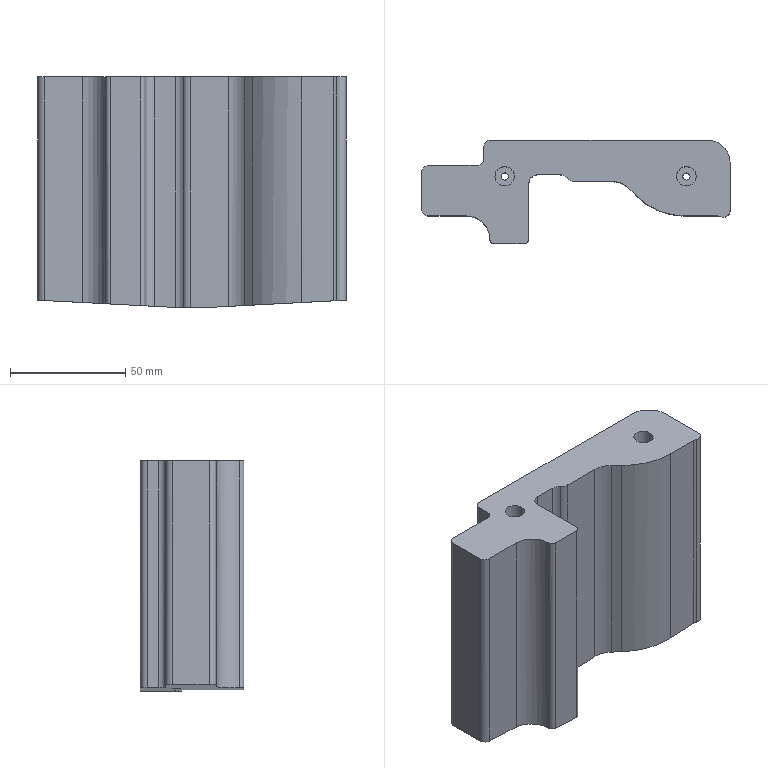Part | STEP file | lll_id238_x_t | 1 solid | 37 faces | box 134 x 45 x 100 mm | volume 341520 mm3 | cylinder 19 | plane 18 | commonest cylinder face diameters 6 x6 3.1 x2 4 x2 8 x2 8.506 x2 20 x2
STEP:
#1=CARTESIAN_POINT('',(1111.,-25.501,-7.5));
#2=VERTEX_POINT('',#1);
#3=CARTESIAN_POINT('',(1111.,-7.5,-7.5));
#4=VERTEX_POINT('',#3);
#5=CARTESIAN_POINT('',(1111.,-7.5,-7.5));
#6=DIRECTION('',(0.,1.,0.));
#7=VECTOR('',#6,1.);
#8=LINE('',#5,#7);
#9=EDGE_CURVE('',#2,#4,#8,.T.);
#10=ORIENTED_EDGE('',*,*,#9,.F.);
#11=CARTESIAN_POINT('',(1100.313,-25.498,-7.5));
#12=VERTEX_POINT('',#11);
#13=CARTESIAN_POINT('',(1065.507,-25.488,-7.5));
#14=DIRECTION('',(-1.,0.0002888,0.));
#15=VECTOR('',#14,1.);
#16=LINE('',#13,#15);
#17=EDGE_CURVE('',#2,#12,#16,.T.);
#18=ORIENTED_EDGE('',*,*,#17,.T.);
#19=CARTESIAN_POINT('',(1097.128,-23.983,-7.5));
#20=VERTEX_POINT('',#19);
#21=CARTESIAN_POINT('',(1100.299,-21.422,-7.5));
#22=DIRECTION('',(0.,0.,1.));
#23=DIRECTION('',(1.,0.,0.));
#24=AXIS2_PLACEMENT_3D('',#21,#22,#23);
#25=CIRCLE('',#24,4.076);
#26=EDGE_CURVE('',#20,#12,#25,.T.);
#27=ORIENTED_EDGE('',*,*,#26,.F.);
#28=CARTESIAN_POINT('',(1094.017,-22.497,-7.5));
#29=VERTEX_POINT('',#28);
#30=CARTESIAN_POINT('',(1094.016,-26.497,-7.5));
#31=DIRECTION('',(0.,0.,-1.));
#32=DIRECTION('',(1.,0.,0.));
#33=AXIS2_PLACEMENT_3D('',#30,#31,#32);
#34=CIRCLE('',#33,4.);
#35=EDGE_CURVE('',#29,#20,#34,.T.);
#36=ORIENTED_EDGE('',*,*,#35,.F.);
#37=CARTESIAN_POINT('',(1091.,-22.496,-7.5));
#38=VERTEX_POINT('',#37);
#39=CARTESIAN_POINT('',(1065.505,-22.492,-7.5));
#40=DIRECTION('',(-1.,0.0001728,0.));
#41=VECTOR('',#40,1.);
#42=LINE('',#39,#41);
#43=EDGE_CURVE('',#29,#38,#42,.T.);
#44=ORIENTED_EDGE('',*,*,#43,.T.);
#45=CARTESIAN_POINT('',(1091.,-7.5,-7.5));
#46=VERTEX_POINT('',#45);
#47=CARTESIAN_POINT('',(1091.,-7.5,-7.5));
#48=DIRECTION('',(0.,-1.,0.));
#49=VECTOR('',#48,1.);
#50=LINE('',#47,#49);
#51=EDGE_CURVE('',#46,#38,#50,.T.);
#52=ORIENTED_EDGE('',*,*,#51,.F.);
#53=CARTESIAN_POINT('',(1065.5,-7.5,-7.5));
#54=DIRECTION('',(-1.,0.,0.));
#55=VECTOR('',#54,1.);
#56=LINE('',#53,#55);
#57=EDGE_CURVE('',#4,#46,#56,.T.);
#58=ORIENTED_EDGE('',*,*,#57,.F.);
#59=EDGE_LOOP('',(#10,#18,#27,#36,#44,#52,#58));
#60=FACE_OUTER_BOUND('',#59,.T.);
#61=CARTESIAN_POINT('',(1065.5,-50.5,-7.5));
#62=DIRECTION('',(0.,0.,1.));
#63=DIRECTION('',(-1.,0.,0.));
#64=AXIS2_PLACEMENT_3D('',#61,#62,#63);
#65=PLANE('',#64);
#66=ADVANCED_FACE('',(#60),#65,.F.);
#67=CARTESIAN_POINT('',(1068.45,-23.25,30.747));
#68=VERTEX_POINT('',#67);
#69=CARTESIAN_POINT('',(1070.,-23.25,30.747));
#70=DIRECTION('',(0.,0.,1.));
#71=DIRECTION('',(-1.,0.,0.));
#72=AXIS2_PLACEMENT_3D('',#69,#70,#71);
#73=CIRCLE('',#72,1.55);
#74=EDGE_CURVE('',#68,#68,#73,.T.);
#75=ORIENTED_EDGE('',*,*,#74,.T.);
#76=EDGE_LOOP('',(#75));
#77=FACE_BOUND('',#76,.T.);
#78=CARTESIAN_POINT('',(1071.55,-23.25,-6.476));
#79=VERTEX_POINT('',#78);
#80=CARTESIAN_POINT('',(1070.,-23.25,-6.395));
#81=DIRECTION('',(-0.05256,0.,-0.9986));
#82=DIRECTION('',(0.9986,0.,-0.05256));
#83=AXIS2_PLACEMENT_3D('',#80,#81,#82);
#84=ELLIPSE('',#83,1.552,1.55);
#85=EDGE_CURVE('',#79,#79,#84,.T.);
#86=ORIENTED_EDGE('',*,*,#85,.T.);
#87=EDGE_LOOP('',(#86));
#88=FACE_BOUND('',#87,.T.);
#89=CARTESIAN_POINT('',(1070.,-23.25,37.747));
#90=DIRECTION('',(0.,0.,-1.));
#91=DIRECTION('',(-1.,0.,0.));
#92=AXIS2_PLACEMENT_3D('',#89,#90,#91);
#93=CYLINDRICAL_SURFACE('',#92,1.55);
#94=ADVANCED_FACE('',(#77,#88),#93,.F.);
#95=CARTESIAN_POINT('',(1147.45,-23.25,30.747));
#96=VERTEX_POINT('',#95);
#97=CARTESIAN_POINT('',(1149.,-23.25,30.747));
#98=DIRECTION('',(0.,0.,1.));
#99=DIRECTION('',(-1.,0.,0.));
#100=AXIS2_PLACEMENT_3D('',#97,#98,#99);
#101=CIRCLE('',#100,1.55);
#102=EDGE_CURVE('',#96,#96,#101,.T.);
#103=ORIENTED_EDGE('',*,*,#102,.T.);
#104=EDGE_LOOP('',(#103));
#105=FACE_BOUND('',#104,.T.);
#106=CARTESIAN_POINT('',(1147.45,-23.25,-5.582));
#107=VERTEX_POINT('',#106);
#108=CARTESIAN_POINT('',(1149.,-23.25,-5.5));
#109=DIRECTION('',(0.05256,0.,-0.9986));
#110=DIRECTION('',(-0.9986,0.,-0.05256));
#111=AXIS2_PLACEMENT_3D('',#108,#109,#110);
#112=ELLIPSE('',#111,1.552,1.55);
#113=EDGE_CURVE('',#107,#107,#112,.T.);
#114=ORIENTED_EDGE('',*,*,#113,.T.);
#115=EDGE_LOOP('',(#114));
#116=FACE_BOUND('',#115,.T.);
#117=CARTESIAN_POINT('',(1149.,-23.25,37.747));
#118=DIRECTION('',(0.,0.,-1.));
#119=DIRECTION('',(-1.,0.,0.));
#120=AXIS2_PLACEMENT_3D('',#117,#118,#119);
#121=CYLINDRICAL_SURFACE('',#120,1.55);
#122=ADVANCED_FACE('',(#105,#116),#121,.F.);
#123=CARTESIAN_POINT('',(1116.863,-25.503,92.5));
#124=VERTEX_POINT('',#123);
#125=CARTESIAN_POINT('',(1100.313,-25.498,92.5));
#126=VERTEX_POINT('',#125);
#127=CARTESIAN_POINT('',(1065.507,-25.488,92.5));
#128=DIRECTION('',(-1.,0.0002888,0.));
#129=VECTOR('',#128,1.);
#130=LINE('',#127,#129);
#131=EDGE_CURVE('',#124,#126,#130,.T.);
#132=ORIENTED_EDGE('',*,*,#131,.F.);
#133=CARTESIAN_POINT('',(1123.932,-28.432,92.5));
#134=VERTEX_POINT('',#133);
#135=CARTESIAN_POINT('',(1116.86,-35.503,92.5));
#136=DIRECTION('',(0.,0.,1.));
#137=DIRECTION('',(1.,0.,0.));
#138=AXIS2_PLACEMENT_3D('',#135,#136,#137);
#139=CIRCLE('',#138,10.);
#140=EDGE_CURVE('',#134,#124,#139,.T.);
#141=ORIENTED_EDGE('',*,*,#140,.F.);
#142=CARTESIAN_POINT('',(1127.213,-31.713,92.5));
#143=VERTEX_POINT('',#142);
#144=CARTESIAN_POINT('',(1105.75,-10.25,92.5));
#145=DIRECTION('',(0.7071,-0.7071,0.));
#146=VECTOR('',#145,1.);
#147=LINE('',#144,#146);
#148=EDGE_CURVE('',#134,#143,#147,.T.);
#149=ORIENTED_EDGE('',*,*,#148,.T.);
#150=CARTESIAN_POINT('',(1148.426,-40.5,92.5));
#151=VERTEX_POINT('',#150);
#152=CARTESIAN_POINT('',(1148.426,-10.502,92.5));
#153=DIRECTION('',(0.,0.,1.));
#154=DIRECTION('',(1.,0.,0.));
#155=AXIS2_PLACEMENT_3D('',#152,#153,#154);
#156=CIRCLE('',#155,29.998);
#157=EDGE_CURVE('',#143,#151,#156,.T.);
#158=ORIENTED_EDGE('',*,*,#157,.T.);
#159=CARTESIAN_POINT('',(1162.602,-40.5,92.5));
#160=VERTEX_POINT('',#159);
#161=CARTESIAN_POINT('',(1065.5,-40.5,92.5));
#162=DIRECTION('',(1.,0.,0.));
#163=VECTOR('',#162,1.);
#164=LINE('',#161,#163);
#165=EDGE_CURVE('',#151,#160,#164,.T.);
#166=ORIENTED_EDGE('',*,*,#165,.T.);
#167=CARTESIAN_POINT('',(1163.801,-40.75,92.5));
#168=VERTEX_POINT('',#167);
#169=CARTESIAN_POINT('',(1162.602,-43.5,92.5));
#170=DIRECTION('',(0.,0.,-1.));
#171=DIRECTION('',(1.,0.,0.));
#172=AXIS2_PLACEMENT_3D('',#169,#170,#171);
#173=CIRCLE('',#172,3.);
#174=EDGE_CURVE('',#160,#168,#173,.T.);
#175=ORIENTED_EDGE('',*,*,#174,.T.);
#176=CARTESIAN_POINT('',(1168.,-38.,92.5));
#177=VERTEX_POINT('',#176);
#178=CARTESIAN_POINT('',(1165.,-38.,92.5));
#179=DIRECTION('',(0.,0.,1.));
#180=DIRECTION('',(1.,0.,0.));
#181=AXIS2_PLACEMENT_3D('',#178,#179,#180);
#182=CIRCLE('',#181,3.);
#183=EDGE_CURVE('',#168,#177,#182,.T.);
#184=ORIENTED_EDGE('',*,*,#183,.T.);
#185=CARTESIAN_POINT('',(1168.,-17.5,92.5));
#186=VERTEX_POINT('',#185);
#187=CARTESIAN_POINT('',(1168.,-50.5,92.5));
#188=DIRECTION('',(0.,-1.,0.));
#189=VECTOR('',#188,1.);
#190=LINE('',#187,#189);
#191=EDGE_CURVE('',#186,#177,#190,.T.);
#192=ORIENTED_EDGE('',*,*,#191,.F.);
#193=CARTESIAN_POINT('',(1158.,-7.5,92.5));
#194=VERTEX_POINT('',#193);
#195=CARTESIAN_POINT('',(1158.,-17.5,92.5));
#196=DIRECTION('',(0.,0.,1.));
#197=DIRECTION('',(1.,0.,0.));
#198=AXIS2_PLACEMENT_3D('',#195,#196,#197);
#199=CIRCLE('',#198,10.);
#200=EDGE_CURVE('',#186,#194,#199,.T.);
#201=ORIENTED_EDGE('',*,*,#200,.T.);
#202=CARTESIAN_POINT('',(1064.,-7.5,92.5));
#203=VERTEX_POINT('',#202);
#204=CARTESIAN_POINT('',(1065.5,-7.5,92.5));
#205=DIRECTION('',(-1.,0.,0.));
#206=VECTOR('',#205,1.);
#207=LINE('',#204,#206);
#208=EDGE_CURVE('',#194,#203,#207,.T.);
#209=ORIENTED_EDGE('',*,*,#208,.T.);
#210=CARTESIAN_POINT('',(1061.,-10.5,92.5));
#211=VERTEX_POINT('',#210);
#212=CARTESIAN_POINT('',(1064.,-10.5,92.5));
#213=DIRECTION('',(0.,0.,-1.));
#214=DIRECTION('',(1.,0.,0.));
#215=AXIS2_PLACEMENT_3D('',#212,#213,#214);
#216=CIRCLE('',#215,3.);
#217=EDGE_CURVE('',#211,#203,#216,.T.);
#218=ORIENTED_EDGE('',*,*,#217,.F.);
#219=CARTESIAN_POINT('',(1061.,-15.5,92.5));
#220=VERTEX_POINT('',#219);
#221=CARTESIAN_POINT('',(1061.,-50.5,92.5));
#222=DIRECTION('',(0.,1.,0.));
#223=VECTOR('',#222,1.);
#224=LINE('',#221,#223);
#225=EDGE_CURVE('',#220,#211,#224,.T.);
#226=ORIENTED_EDGE('',*,*,#225,.F.);
#227=CARTESIAN_POINT('',(1058.,-18.5,92.5));
#228=VERTEX_POINT('',#227);
#229=CARTESIAN_POINT('',(1058.,-15.5,92.5));
#230=DIRECTION('',(0.,0.,-1.));
#231=DIRECTION('',(1.,0.,0.));
#232=AXIS2_PLACEMENT_3D('',#229,#230,#231);
#233=CIRCLE('',#232,3.);
#234=EDGE_CURVE('',#220,#228,#233,.T.);
#235=ORIENTED_EDGE('',*,*,#234,.T.);
#236=CARTESIAN_POINT('',(1037.,-18.5,92.5));
#237=VERTEX_POINT('',#236);
#238=CARTESIAN_POINT('',(1065.5,-18.5,92.5));
#239=DIRECTION('',(1.,0.,0.));
#240=VECTOR('',#239,1.);
#241=LINE('',#238,#240);
#242=EDGE_CURVE('',#237,#228,#241,.T.);
#243=ORIENTED_EDGE('',*,*,#242,.F.);
#244=CARTESIAN_POINT('',(1034.,-21.5,92.5));
#245=VERTEX_POINT('',#244);
#246=CARTESIAN_POINT('',(1037.,-21.5,92.5));
#247=DIRECTION('',(0.,0.,1.));
#248=DIRECTION('',(1.,0.,0.));
#249=AXIS2_PLACEMENT_3D('',#246,#247,#248);
#250=CIRCLE('',#249,3.);
#251=EDGE_CURVE('',#237,#245,#250,.T.);
#252=ORIENTED_EDGE('',*,*,#251,.T.);
#253=CARTESIAN_POINT('',(1034.,-37.5,92.5));
#254=VERTEX_POINT('',#253);
#255=CARTESIAN_POINT('',(1034.,-50.5,92.5));
#256=DIRECTION('',(0.,1.,0.));
#257=VECTOR('',#256,1.);
#258=LINE('',#255,#257);
#259=EDGE_CURVE('',#254,#245,#258,.T.);
#260=ORIENTED_EDGE('',*,*,#259,.F.);
#261=CARTESIAN_POINT('',(1037.,-40.5,92.5));
#262=VERTEX_POINT('',#261);
#263=CARTESIAN_POINT('',(1037.,-37.5,92.5));
#264=DIRECTION('',(0.,0.,-1.));
#265=DIRECTION('',(1.,0.,0.));
#266=AXIS2_PLACEMENT_3D('',#263,#264,#265);
#267=CIRCLE('',#266,3.);
#268=EDGE_CURVE('',#262,#254,#267,.T.);
#269=ORIENTED_EDGE('',*,*,#268,.F.);
#270=CARTESIAN_POINT('',(1053.5,-40.5,92.5));
#271=VERTEX_POINT('',#270);
#272=CARTESIAN_POINT('',(1065.5,-40.5,92.5));
#273=DIRECTION('',(1.,0.,0.));
#274=VECTOR('',#273,1.);
#275=LINE('',#272,#274);
#276=EDGE_CURVE('',#262,#271,#275,.T.);
#277=ORIENTED_EDGE('',*,*,#276,.T.);
#278=CARTESIAN_POINT('',(1063.5,-50.5,92.5));
#279=VERTEX_POINT('',#278);
#280=CARTESIAN_POINT('',(1053.499,-50.501,92.5));
#281=DIRECTION('',(0.,0.,-1.));
#282=DIRECTION('',(1.,0.,0.));
#283=AXIS2_PLACEMENT_3D('',#280,#281,#282);
#284=CIRCLE('',#283,10.001);
#285=EDGE_CURVE('',#271,#279,#284,.T.);
#286=ORIENTED_EDGE('',*,*,#285,.T.);
#287=CARTESIAN_POINT('',(1065.5,-52.5,92.5));
#288=VERTEX_POINT('',#287);
#289=CARTESIAN_POINT('',(1065.5,-50.5,92.5));
#290=DIRECTION('',(0.,0.,1.));
#291=DIRECTION('',(1.,0.,0.));
#292=AXIS2_PLACEMENT_3D('',#289,#290,#291);
#293=CIRCLE('',#292,2.);
#294=EDGE_CURVE('',#279,#288,#293,.T.);
#295=ORIENTED_EDGE('',*,*,#294,.T.);
#296=CARTESIAN_POINT('',(1078.51,-52.5,92.5));
#297=VERTEX_POINT('',#296);
#298=CARTESIAN_POINT('',(1065.5,-52.5,92.5));
#299=DIRECTION('',(-1.,0.,0.));
#300=VECTOR('',#299,1.);
#301=LINE('',#298,#300);
#302=EDGE_CURVE('',#297,#288,#301,.T.);
#303=ORIENTED_EDGE('',*,*,#302,.F.);
#304=CARTESIAN_POINT('',(1080.51,-50.5,92.5));
#305=VERTEX_POINT('',#304);
#306=CARTESIAN_POINT('',(1078.51,-50.5,92.5));
#307=DIRECTION('',(0.,0.,-1.));
#308=DIRECTION('',(1.,0.,0.));
#309=AXIS2_PLACEMENT_3D('',#306,#307,#308);
#310=CIRCLE('',#309,2.);
#311=EDGE_CURVE('',#305,#297,#310,.T.);
#312=ORIENTED_EDGE('',*,*,#311,.F.);
#313=CARTESIAN_POINT('',(1080.512,-26.495,92.5));
#314=VERTEX_POINT('',#313);
#315=CARTESIAN_POINT('',(1080.51,-50.501,92.5));
#316=DIRECTION('',(0.00006142,1.,0.));
#317=VECTOR('',#316,1.);
#318=LINE('',#315,#317);
#319=EDGE_CURVE('',#305,#314,#318,.T.);
#320=ORIENTED_EDGE('',*,*,#319,.T.);
#321=CARTESIAN_POINT('',(1084.513,-22.495,92.5));
#322=VERTEX_POINT('',#321);
#323=CARTESIAN_POINT('',(1084.512,-26.495,92.5));
#324=DIRECTION('',(0.,0.,1.));
#325=DIRECTION('',(1.,0.,0.));
#326=AXIS2_PLACEMENT_3D('',#323,#324,#325);
#327=CIRCLE('',#326,4.);
#328=EDGE_CURVE('',#322,#314,#327,.T.);
#329=ORIENTED_EDGE('',*,*,#328,.F.);
#330=CARTESIAN_POINT('',(1094.017,-22.497,92.5));
#331=VERTEX_POINT('',#330);
#332=CARTESIAN_POINT('',(1065.505,-22.492,92.5));
#333=DIRECTION('',(1.,-0.0001728,0.));
#334=VECTOR('',#333,1.);
#335=LINE('',#332,#334);
#336=EDGE_CURVE('',#322,#331,#335,.T.);
#337=ORIENTED_EDGE('',*,*,#336,.T.);
#338=CARTESIAN_POINT('',(1097.128,-23.983,92.5));
#339=VERTEX_POINT('',#338);
#340=CARTESIAN_POINT('',(1094.016,-26.497,92.5));
#341=DIRECTION('',(0.,0.,1.));
#342=DIRECTION('',(1.,0.,0.));
#343=AXIS2_PLACEMENT_3D('',#340,#341,#342);
#344=CIRCLE('',#343,4.);
#345=EDGE_CURVE('',#339,#331,#344,.T.);
#346=ORIENTED_EDGE('',*,*,#345,.F.);
#347=CARTESIAN_POINT('',(1100.299,-21.422,92.5));
#348=DIRECTION('',(0.,0.,1.));
#349=DIRECTION('',(1.,0.,0.));
#350=AXIS2_PLACEMENT_3D('',#347,#348,#349);
#351=CIRCLE('',#350,4.076);
#352=EDGE_CURVE('',#339,#126,#351,.T.);
#353=ORIENTED_EDGE('',*,*,#352,.T.);
#354=EDGE_LOOP('',(#132,#141,#149,#158,#166,#175,#184,#192,#201,#209,#218,#226,#235,#243,#252,#260,#269,#277,#286,#295,#303,#312,#320,#329,#337,#346,#353));
#355=FACE_BOUND('',#354,.T.);
#356=CARTESIAN_POINT('',(1153.253,-23.25,92.5));
#357=VERTEX_POINT('',#356);
#358=CARTESIAN_POINT('',(1149.,-23.25,92.5));
#359=DIRECTION('',(0.,0.,-1.));
#360=DIRECTION('',(1.,0.,0.));
#361=AXIS2_PLACEMENT_3D('',#358,#359,#360);
#362=CIRCLE('',#361,4.253);
#363=EDGE_CURVE('',#357,#357,#362,.T.);
#364=ORIENTED_EDGE('',*,*,#363,.T.);
#365=EDGE_LOOP('',(#364));
#366=FACE_BOUND('',#365,.T.);
#367=CARTESIAN_POINT('',(1074.253,-23.25,92.5));
#368=VERTEX_POINT('',#367);
#369=CARTESIAN_POINT('',(1070.,-23.25,92.5));
#370=DIRECTION('',(0.,0.,-1.));
#371=DIRECTION('',(1.,0.,0.));
#372=AXIS2_PLACEMENT_3D('',#369,#370,#371);
#373=CIRCLE('',#372,4.253);
#374=EDGE_CURVE('',#368,#368,#373,.T.);
#375=ORIENTED_EDGE('',*,*,#374,.T.);
#376=EDGE_LOOP('',(#375));
#377=FACE_BOUND('',#376,.T.);
#378=CARTESIAN_POINT('',(1065.5,-50.5,92.5));
#379=DIRECTION('',(0.,0.,1.));
#380=DIRECTION('',(-1.,0.,0.));
#381=AXIS2_PLACEMENT_3D('',#378,#379,#380);
#382=PLANE('',#381);
#383=ADVANCED_FACE('',(#355,#366,#377),#382,.T.);
#384=ORIENTED_EDGE('',*,*,#363,.F.);
#385=EDGE_LOOP('',(#384));
#386=FACE_BOUND('',#385,.T.);
#387=CARTESIAN_POINT('',(1144.747,-23.25,30.747));
#388=VERTEX_POINT('',#387);
#389=CARTESIAN_POINT('',(1149.,-23.25,30.747));
#390=DIRECTION('',(0.,0.,-1.));
#391=DIRECTION('',(-1.,0.,0.));
#392=AXIS2_PLACEMENT_3D('',#389,#390,#391);
#393=CIRCLE('',#392,4.253);
#394=EDGE_CURVE('',#388,#388,#393,.T.);
#395=ORIENTED_EDGE('',*,*,#394,.T.);
#396=EDGE_LOOP('',(#395));
#397=FACE_BOUND('',#396,.T.);
#398=CARTESIAN_POINT('',(1149.,-23.25,94.5));
#399=DIRECTION('',(0.,0.,-1.));
#400=DIRECTION('',(1.,0.,0.));
#401=AXIS2_PLACEMENT_3D('',#398,#399,#400);
#402=CYLINDRICAL_SURFACE('',#401,4.253);
#403=ADVANCED_FACE('',(#386,#397),#402,.F.);
#404=ORIENTED_EDGE('',*,*,#374,.F.);
#405=EDGE_LOOP('',(#404));
#406=FACE_BOUND('',#405,.T.);
#407=CARTESIAN_POINT('',(1065.747,-23.25,30.747));
#408=VERTEX_POINT('',#407);
#409=CARTESIAN_POINT('',(1070.,-23.25,30.747));
#410=DIRECTION('',(0.,0.,-1.));
#411=DIRECTION('',(-1.,0.,0.));
#412=AXIS2_PLACEMENT_3D('',#409,#410,#411);
#413=CIRCLE('',#412,4.253);
#414=EDGE_CURVE('',#408,#408,#413,.T.);
#415=ORIENTED_EDGE('',*,*,#414,.T.);
#416=EDGE_LOOP('',(#415));
#417=FACE_BOUND('',#416,.T.);
#418=CARTESIAN_POINT('',(1070.,-23.25,94.5));
#419=DIRECTION('',(0.,0.,-1.));
#420=DIRECTION('',(1.,0.,0.));
#421=AXIS2_PLACEMENT_3D('',#418,#419,#420);
#422=CYLINDRICAL_SURFACE('',#421,4.253);
#423=ADVANCED_FACE('',(#406,#417),#422,.F.);
#424=CARTESIAN_POINT('',(1116.863,-25.503,-7.191));
#425=VERTEX_POINT('',#424);
#426=CARTESIAN_POINT('',(1110.995,-25.501,-7.5));
#427=DIRECTION('',(-0.9986,0.0002884,-0.05256));
#428=VECTOR('',#427,1.);
#429=LINE('',#426,#428);
#430=EDGE_CURVE('',#425,#2,#429,.T.);
#431=ORIENTED_EDGE('',*,*,#430,.T.);
#432=ORIENTED_EDGE('',*,*,#9,.T.);
#433=CARTESIAN_POINT('',(1158.,-7.5,-5.026));
#434=VERTEX_POINT('',#433);
#435=CARTESIAN_POINT('',(1111.,-7.5,-7.5));
#436=DIRECTION('',(0.9986,0.,0.05256));
#437=VECTOR('',#436,1.);
#438=LINE('',#435,#437);
#439=EDGE_CURVE('',#4,#434,#438,.T.);
#440=ORIENTED_EDGE('',*,*,#439,.T.);
#441=CARTESIAN_POINT('',(1168.,-17.5,-4.5));
#442=VERTEX_POINT('',#441);
#443=CARTESIAN_POINT('',(1158.,-17.5,-5.026));
#444=DIRECTION('',(-0.05256,0.,0.9986));
#445=DIRECTION('',(0.9986,0.,0.05256));
#446=AXIS2_PLACEMENT_3D('',#443,#444,#445);
#447=ELLIPSE('',#446,10.014,10.);
#448=EDGE_CURVE('',#442,#434,#447,.T.);
#449=ORIENTED_EDGE('',*,*,#448,.F.);
#450=CARTESIAN_POINT('',(1168.,-38.,-4.5));
#451=VERTEX_POINT('',#450);
#452=CARTESIAN_POINT('',(1168.,-7.5,-4.5));
#453=DIRECTION('',(0.,-1.,0.));
#454=VECTOR('',#453,1.);
#455=LINE('',#452,#454);
#456=EDGE_CURVE('',#442,#451,#455,.T.);
#457=ORIENTED_EDGE('',*,*,#456,.T.);
#458=CARTESIAN_POINT('',(1163.801,-40.75,-4.721));
#459=VERTEX_POINT('',#458);
#460=CARTESIAN_POINT('',(1165.,-38.,-4.658));
#461=DIRECTION('',(-0.05256,0.,0.9986));
#462=DIRECTION('',(0.9986,0.,0.05256));
#463=AXIS2_PLACEMENT_3D('',#460,#461,#462);
#464=ELLIPSE('',#463,3.004,3.);
#465=EDGE_CURVE('',#459,#451,#464,.T.);
#466=ORIENTED_EDGE('',*,*,#465,.F.);
#467=CARTESIAN_POINT('',(1162.602,-40.5,-4.784));
#468=VERTEX_POINT('',#467);
#469=CARTESIAN_POINT('',(1162.602,-43.5,-4.784));
#470=DIRECTION('',(0.05256,0.,-0.9986));
#471=DIRECTION('',(0.9986,0.,0.05256));
#472=AXIS2_PLACEMENT_3D('',#469,#470,#471);
#473=ELLIPSE('',#472,3.004,3.);
#474=EDGE_CURVE('',#468,#459,#473,.T.);
#475=ORIENTED_EDGE('',*,*,#474,.F.);
#476=CARTESIAN_POINT('',(1148.426,-40.5,-5.53));
#477=VERTEX_POINT('',#476);
#478=CARTESIAN_POINT('',(1111.,-40.5,-7.5));
#479=DIRECTION('',(-0.9986,0.,-0.05256));
#480=VECTOR('',#479,1.);
#481=LINE('',#478,#480);
#482=EDGE_CURVE('',#468,#477,#481,.T.);
#483=ORIENTED_EDGE('',*,*,#482,.T.);
#484=CARTESIAN_POINT('',(1127.213,-31.713,-6.647));
#485=VERTEX_POINT('',#484);
#486=CARTESIAN_POINT('',(1148.426,-10.502,-5.53));
#487=DIRECTION('',(0.05256,0.,-0.9986));
#488=DIRECTION('',(0.9986,0.,0.05256));
#489=AXIS2_PLACEMENT_3D('',#486,#487,#488);
#490=ELLIPSE('',#489,30.039,29.998);
#491=EDGE_CURVE('',#477,#485,#490,.T.);
#492=ORIENTED_EDGE('',*,*,#491,.T.);
#493=CARTESIAN_POINT('',(1123.932,-28.432,-6.819));
#494=VERTEX_POINT('',#493);
#495=CARTESIAN_POINT('',(1107.006,-11.506,-7.71));
#496=DIRECTION('',(0.7066,-0.7066,0.03719));
#497=VECTOR('',#496,1.);
#498=LINE('',#495,#497);
#499=EDGE_CURVE('',#494,#485,#498,.T.);
#500=ORIENTED_EDGE('',*,*,#499,.F.);
#501=CARTESIAN_POINT('',(1116.86,-35.503,-7.192));
#502=DIRECTION('',(-0.05256,0.,0.9986));
#503=DIRECTION('',(0.9986,0.,0.05256));
#504=AXIS2_PLACEMENT_3D('',#501,#502,#503);
#505=ELLIPSE('',#504,10.014,10.);
#506=EDGE_CURVE('',#494,#425,#505,.T.);
#507=ORIENTED_EDGE('',*,*,#506,.T.);
#508=EDGE_LOOP('',(#431,#432,#440,#449,#457,#466,#475,#483,#492,#500,#507));
#509=FACE_BOUND('',#508,.T.);
#510=ORIENTED_EDGE('',*,*,#113,.F.);
#511=EDGE_LOOP('',(#510));
#512=FACE_BOUND('',#511,.T.);
#513=CARTESIAN_POINT('',(1111.,-7.5,-7.5));
#514=DIRECTION('',(0.05256,0.,-0.9986));
#515=DIRECTION('',(-0.9986,0.,-0.05256));
#516=AXIS2_PLACEMENT_3D('',#513,#514,#515);
#517=PLANE('',#516);
#518=ADVANCED_FACE('',(#509,#512),#517,.T.);
#519=CARTESIAN_POINT('',(1084.513,-22.495,-7.159));
#520=VERTEX_POINT('',#519);
#521=CARTESIAN_POINT('',(1090.997,-22.496,-7.5));
#522=DIRECTION('',(0.9986,-0.0001725,-0.05256));
#523=VECTOR('',#522,1.);
#524=LINE('',#521,#523);
#525=EDGE_CURVE('',#520,#38,#524,.T.);
#526=ORIENTED_EDGE('',*,*,#525,.F.);
#527=CARTESIAN_POINT('',(1080.512,-26.495,-6.948));
#528=VERTEX_POINT('',#527);
#529=CARTESIAN_POINT('',(1084.512,-26.495,-7.159));
#530=DIRECTION('',(0.05256,0.,0.9986));
#531=DIRECTION('',(-0.9986,0.,0.05256));
#532=AXIS2_PLACEMENT_3D('',#529,#530,#531);
#533=ELLIPSE('',#532,4.006,4.);
#534=EDGE_CURVE('',#520,#528,#533,.T.);
#535=ORIENTED_EDGE('',*,*,#534,.T.);
#536=CARTESIAN_POINT('',(1080.51,-50.5,-6.948));
#537=VERTEX_POINT('',#536);
#538=CARTESIAN_POINT('',(1080.513,-7.499,-6.948));
#539=DIRECTION('',(0.00006142,1.,-0.000003233));
#540=VECTOR('',#539,1.);
#541=LINE('',#538,#540);
#542=EDGE_CURVE('',#537,#528,#541,.T.);
#543=ORIENTED_EDGE('',*,*,#542,.F.);
#544=CARTESIAN_POINT('',(1078.51,-52.5,-6.843));
#545=VERTEX_POINT('',#544);
#546=CARTESIAN_POINT('',(1078.51,-50.5,-6.843));
#547=DIRECTION('',(-0.05256,0.,-0.9986));
#548=DIRECTION('',(-0.9986,0.,0.05256));
#549=AXIS2_PLACEMENT_3D('',#546,#547,#548);
#550=ELLIPSE('',#549,2.003,2.);
#551=EDGE_CURVE('',#537,#545,#550,.T.);
#552=ORIENTED_EDGE('',*,*,#551,.T.);
#553=CARTESIAN_POINT('',(1065.5,-52.5,-6.158));
#554=VERTEX_POINT('',#553);
#555=CARTESIAN_POINT('',(1091.,-52.5,-7.5));
#556=DIRECTION('',(-0.9986,0.,0.05256));
#557=VECTOR('',#556,1.);
#558=LINE('',#555,#557);
#559=EDGE_CURVE('',#545,#554,#558,.T.);
#560=ORIENTED_EDGE('',*,*,#559,.T.);
#561=CARTESIAN_POINT('',(1063.5,-50.5,-6.053));
#562=VERTEX_POINT('',#561);
#563=CARTESIAN_POINT('',(1065.5,-50.5,-6.158));
#564=DIRECTION('',(0.05256,0.,0.9986));
#565=DIRECTION('',(-0.9986,0.,0.05256));
#566=AXIS2_PLACEMENT_3D('',#563,#564,#565);
#567=ELLIPSE('',#566,2.003,2.);
#568=EDGE_CURVE('',#562,#554,#567,.T.);
#569=ORIENTED_EDGE('',*,*,#568,.F.);
#570=CARTESIAN_POINT('',(1053.5,-40.5,-5.526));
#571=VERTEX_POINT('',#570);
#572=CARTESIAN_POINT('',(1053.499,-50.501,-5.526));
#573=DIRECTION('',(-0.05256,0.,-0.9986));
#574=DIRECTION('',(-0.9986,0.,0.05256));
#575=AXIS2_PLACEMENT_3D('',#572,#573,#574);
#576=ELLIPSE('',#575,10.014,10.001);
#577=EDGE_CURVE('',#571,#562,#576,.T.);
#578=ORIENTED_EDGE('',*,*,#577,.F.);
#579=CARTESIAN_POINT('',(1037.,-40.5,-4.658));
#580=VERTEX_POINT('',#579);
#581=CARTESIAN_POINT('',(1091.,-40.5,-7.5));
#582=DIRECTION('',(-0.9986,0.,0.05256));
#583=VECTOR('',#582,1.);
#584=LINE('',#581,#583);
#585=EDGE_CURVE('',#571,#580,#584,.T.);
#586=ORIENTED_EDGE('',*,*,#585,.T.);
#587=CARTESIAN_POINT('',(1034.,-37.5,-4.5));
#588=VERTEX_POINT('',#587);
#589=CARTESIAN_POINT('',(1037.,-37.5,-4.658));
#590=DIRECTION('',(-0.05256,0.,-0.9986));
#591=DIRECTION('',(-0.9986,0.,0.05256));
#592=AXIS2_PLACEMENT_3D('',#589,#590,#591);
#593=ELLIPSE('',#592,3.004,3.);
#594=EDGE_CURVE('',#580,#588,#593,.T.);
#595=ORIENTED_EDGE('',*,*,#594,.T.);
#596=CARTESIAN_POINT('',(1034.,-21.5,-4.5));
#597=VERTEX_POINT('',#596);
#598=CARTESIAN_POINT('',(1034.,-7.5,-4.5));
#599=DIRECTION('',(0.,-1.,0.));
#600=VECTOR('',#599,1.);
#601=LINE('',#598,#600);
#602=EDGE_CURVE('',#597,#588,#601,.T.);
#603=ORIENTED_EDGE('',*,*,#602,.F.);
#604=CARTESIAN_POINT('',(1037.,-18.5,-4.658));
#605=VERTEX_POINT('',#604);
#606=CARTESIAN_POINT('',(1037.,-21.5,-4.658));
#607=DIRECTION('',(0.05256,0.,0.9986));
#608=DIRECTION('',(-0.9986,0.,0.05256));
#609=AXIS2_PLACEMENT_3D('',#606,#607,#608);
#610=ELLIPSE('',#609,3.004,3.);
#611=EDGE_CURVE('',#605,#597,#610,.T.);
#612=ORIENTED_EDGE('',*,*,#611,.F.);
#613=CARTESIAN_POINT('',(1058.,-18.5,-5.763));
#614=VERTEX_POINT('',#613);
#615=CARTESIAN_POINT('',(1091.,-18.5,-7.5));
#616=DIRECTION('',(-0.9986,0.,0.05256));
#617=VECTOR('',#616,1.);
#618=LINE('',#615,#617);
#619=EDGE_CURVE('',#614,#605,#618,.T.);
#620=ORIENTED_EDGE('',*,*,#619,.F.);
#621=CARTESIAN_POINT('',(1061.,-15.5,-5.921));
#622=VERTEX_POINT('',#621);
#623=CARTESIAN_POINT('',(1058.,-15.5,-5.763));
#624=DIRECTION('',(-0.05256,0.,-0.9986));
#625=DIRECTION('',(-0.9986,0.,0.05256));
#626=AXIS2_PLACEMENT_3D('',#623,#624,#625);
#627=ELLIPSE('',#626,3.004,3.);
#628=EDGE_CURVE('',#622,#614,#627,.T.);
#629=ORIENTED_EDGE('',*,*,#628,.F.);
#630=CARTESIAN_POINT('',(1061.,-10.5,-5.921));
#631=VERTEX_POINT('',#630);
#632=CARTESIAN_POINT('',(1061.,-7.5,-5.921));
#633=DIRECTION('',(0.,-1.,0.));
#634=VECTOR('',#633,1.);
#635=LINE('',#632,#634);
#636=EDGE_CURVE('',#631,#622,#635,.T.);
#637=ORIENTED_EDGE('',*,*,#636,.F.);
#638=CARTESIAN_POINT('',(1064.,-7.5,-6.079));
#639=VERTEX_POINT('',#638);
#640=CARTESIAN_POINT('',(1064.,-10.5,-6.079));
#641=DIRECTION('',(-0.05256,0.,-0.9986));
#642=DIRECTION('',(-0.9986,0.,0.05256));
#643=AXIS2_PLACEMENT_3D('',#640,#641,#642);
#644=ELLIPSE('',#643,3.004,3.);
#645=EDGE_CURVE('',#631,#639,#644,.T.);
#646=ORIENTED_EDGE('',*,*,#645,.T.);
#647=CARTESIAN_POINT('',(1091.,-7.5,-7.5));
#648=DIRECTION('',(-0.9986,0.,0.05256));
#649=VECTOR('',#648,1.);
#650=LINE('',#647,#649);
#651=EDGE_CURVE('',#46,#639,#650,.T.);
#652=ORIENTED_EDGE('',*,*,#651,.F.);
#653=ORIENTED_EDGE('',*,*,#51,.T.);
#654=EDGE_LOOP('',(#526,#535,#543,#552,#560,#569,#578,#586,#595,#603,#612,#620,#629,#637,#646,#652,#653));
#655=FACE_BOUND('',#654,.T.);
#656=ORIENTED_EDGE('',*,*,#85,.F.);
#657=EDGE_LOOP('',(#656));
#658=FACE_BOUND('',#657,.T.);
#659=CARTESIAN_POINT('',(1091.,-7.5,-7.5));
#660=DIRECTION('',(-0.05256,0.,-0.9986));
#661=DIRECTION('',(-0.9986,0.,0.05256));
#662=AXIS2_PLACEMENT_3D('',#659,#660,#661);
#663=PLANE('',#662);
#664=ADVANCED_FACE('',(#655,#658),#663,.T.);
#665=ORIENTED_EDGE('',*,*,#414,.F.);
#666=EDGE_LOOP('',(#665));
#667=FACE_BOUND('',#666,.T.);
#668=ORIENTED_EDGE('',*,*,#74,.F.);
#669=EDGE_LOOP('',(#668));
#670=FACE_BOUND('',#669,.T.);
#671=CARTESIAN_POINT('',(1070.,-23.25,30.747));
#672=DIRECTION('',(0.,0.,-1.));
#673=DIRECTION('',(-1.,0.,0.));
#674=AXIS2_PLACEMENT_3D('',#671,#672,#673);
#675=PLANE('',#674);
#676=ADVANCED_FACE('',(#667,#670),#675,.F.);
#677=ORIENTED_EDGE('',*,*,#394,.F.);
#678=EDGE_LOOP('',(#677));
#679=FACE_BOUND('',#678,.T.);
#680=ORIENTED_EDGE('',*,*,#102,.F.);
#681=EDGE_LOOP('',(#680));
#682=FACE_BOUND('',#681,.T.);
#683=CARTESIAN_POINT('',(1149.,-23.25,30.747));
#684=DIRECTION('',(0.,0.,-1.));
#685=DIRECTION('',(-1.,0.,0.));
#686=AXIS2_PLACEMENT_3D('',#683,#684,#685);
#687=PLANE('',#686);
#688=ADVANCED_FACE('',(#679,#682),#687,.F.);
#689=CARTESIAN_POINT('',(1100.313,-25.498,-177.5));
#690=DIRECTION('',(0.,0.,-1.));
#691=VECTOR('',#690,1.);
#692=LINE('',#689,#691);
#693=EDGE_CURVE('',#126,#12,#692,.T.);
#694=ORIENTED_EDGE('',*,*,#693,.F.);
#695=ORIENTED_EDGE('',*,*,#352,.F.);
#696=CARTESIAN_POINT('',(1097.128,-23.983,-177.5));
#697=DIRECTION('',(0.,0.,-1.));
#698=VECTOR('',#697,1.);
#699=LINE('',#696,#698);
#700=EDGE_CURVE('',#339,#20,#699,.T.);
#701=ORIENTED_EDGE('',*,*,#700,.T.);
#702=ORIENTED_EDGE('',*,*,#26,.T.);
#703=EDGE_LOOP('',(#694,#695,#701,#702));
#704=FACE_OUTER_BOUND('',#703,.T.);
#705=CARTESIAN_POINT('',(1100.299,-21.422,-177.5));
#706=DIRECTION('',(0.,0.,1.));
#707=DIRECTION('',(1.,0.,0.));
#708=AXIS2_PLACEMENT_3D('',#705,#706,#707);
#709=CYLINDRICAL_SURFACE('',#708,4.076);
#710=ADVANCED_FACE('',(#704),#709,.T.);
#711=ORIENTED_EDGE('',*,*,#700,.F.);
#712=ORIENTED_EDGE('',*,*,#345,.T.);
#713=CARTESIAN_POINT('',(1094.017,-22.497,-177.5));
#714=DIRECTION('',(0.,0.,-1.));
#715=VECTOR('',#714,1.);
#716=LINE('',#713,#715);
#717=EDGE_CURVE('',#331,#29,#716,.T.);
#718=ORIENTED_EDGE('',*,*,#717,.T.);
#719=ORIENTED_EDGE('',*,*,#35,.T.);
#720=EDGE_LOOP('',(#711,#712,#718,#719));
#721=FACE_OUTER_BOUND('',#720,.T.);
#722=CARTESIAN_POINT('',(1094.016,-26.497,-177.5));
#723=DIRECTION('',(0.,0.,1.));
#724=DIRECTION('',(1.,0.,0.));
#725=AXIS2_PLACEMENT_3D('',#722,#723,#724);
#726=CYLINDRICAL_SURFACE('',#725,4.);
#727=ADVANCED_FACE('',(#721),#726,.F.);
#728=ORIENTED_EDGE('',*,*,#131,.T.);
#729=ORIENTED_EDGE('',*,*,#693,.T.);
#730=ORIENTED_EDGE('',*,*,#17,.F.);
#731=ORIENTED_EDGE('',*,*,#430,.F.);
#732=CARTESIAN_POINT('',(1116.863,-25.503,-177.5));
#733=DIRECTION('',(0.,0.,-1.));
#734=VECTOR('',#733,1.);
#735=LINE('',#732,#734);
#736=EDGE_CURVE('',#124,#425,#735,.T.);
#737=ORIENTED_EDGE('',*,*,#736,.F.);
#738=EDGE_LOOP('',(#728,#729,#730,#731,#737));
#739=FACE_OUTER_BOUND('',#738,.T.);
#740=CARTESIAN_POINT('',(1116.863,-25.503,-177.5));
#741=DIRECTION('',(0.0002888,1.,0.));
#742=DIRECTION('',(-1.,0.0002888,0.));
#743=AXIS2_PLACEMENT_3D('',#740,#741,#742);
#744=PLANE('',#743);
#745=ADVANCED_FACE('',(#739),#744,.F.);
#746=ORIENTED_EDGE('',*,*,#336,.F.);
#747=CARTESIAN_POINT('',(1084.513,-22.495,-177.5));
#748=DIRECTION('',(0.,0.,-1.));
#749=VECTOR('',#748,1.);
#750=LINE('',#747,#749);
#751=EDGE_CURVE('',#322,#520,#750,.T.);
#752=ORIENTED_EDGE('',*,*,#751,.T.);
#753=ORIENTED_EDGE('',*,*,#525,.T.);
#754=ORIENTED_EDGE('',*,*,#43,.F.);
#755=ORIENTED_EDGE('',*,*,#717,.F.);
#756=EDGE_LOOP('',(#746,#752,#753,#754,#755));
#757=FACE_OUTER_BOUND('',#756,.T.);
#758=CARTESIAN_POINT('',(1094.017,-22.497,-177.5));
#759=DIRECTION('',(0.0001728,1.,0.));
#760=DIRECTION('',(-1.,0.0001728,0.));
#761=AXIS2_PLACEMENT_3D('',#758,#759,#760);
#762=PLANE('',#761);
#763=ADVANCED_FACE('',(#757),#762,.F.);
#764=ORIENTED_EDGE('',*,*,#328,.T.);
#765=CARTESIAN_POINT('',(1080.512,-26.495,-177.5));
#766=DIRECTION('',(0.,0.,-1.));
#767=VECTOR('',#766,1.);
#768=LINE('',#765,#767);
#769=EDGE_CURVE('',#314,#528,#768,.T.);
#770=ORIENTED_EDGE('',*,*,#769,.T.);
#771=ORIENTED_EDGE('',*,*,#534,.F.);
#772=ORIENTED_EDGE('',*,*,#751,.F.);
#773=EDGE_LOOP('',(#764,#770,#771,#772));
#774=FACE_OUTER_BOUND('',#773,.T.);
#775=CARTESIAN_POINT('',(1084.512,-26.495,-177.5));
#776=DIRECTION('',(0.,0.,1.));
#777=DIRECTION('',(1.,0.,0.));
#778=AXIS2_PLACEMENT_3D('',#775,#776,#777);
#779=CYLINDRICAL_SURFACE('',#778,4.);
#780=ADVANCED_FACE('',(#774),#779,.F.);
#781=ORIENTED_EDGE('',*,*,#319,.F.);
#782=CARTESIAN_POINT('',(1080.51,-50.5,-177.5));
#783=DIRECTION('',(0.,0.,-1.));
#784=VECTOR('',#783,1.);
#785=LINE('',#782,#784);
#786=EDGE_CURVE('',#305,#537,#785,.T.);
#787=ORIENTED_EDGE('',*,*,#786,.T.);
#788=ORIENTED_EDGE('',*,*,#542,.T.);
#789=ORIENTED_EDGE('',*,*,#769,.F.);
#790=EDGE_LOOP('',(#781,#787,#788,#789));
#791=FACE_OUTER_BOUND('',#790,.T.);
#792=CARTESIAN_POINT('',(1080.512,-26.495,-177.5));
#793=DIRECTION('',(-1.,0.00006142,0.));
#794=DIRECTION('',(-0.00006142,-1.,0.));
#795=AXIS2_PLACEMENT_3D('',#792,#793,#794);
#796=PLANE('',#795);
#797=ADVANCED_FACE('',(#791),#796,.F.);
#798=ORIENTED_EDGE('',*,*,#311,.T.);
#799=CARTESIAN_POINT('',(1078.51,-52.5,-177.5));
#800=DIRECTION('',(0.,0.,-1.));
#801=VECTOR('',#800,1.);
#802=LINE('',#799,#801);
#803=EDGE_CURVE('',#297,#545,#802,.T.);
#804=ORIENTED_EDGE('',*,*,#803,.T.);
#805=ORIENTED_EDGE('',*,*,#551,.F.);
#806=ORIENTED_EDGE('',*,*,#786,.F.);
#807=EDGE_LOOP('',(#798,#804,#805,#806));
#808=FACE_OUTER_BOUND('',#807,.T.);
#809=CARTESIAN_POINT('',(1078.51,-50.5,-177.5));
#810=DIRECTION('',(0.,0.,1.));
#811=DIRECTION('',(1.,0.,0.));
#812=AXIS2_PLACEMENT_3D('',#809,#810,#811);
#813=CYLINDRICAL_SURFACE('',#812,2.);
#814=ADVANCED_FACE('',(#808),#813,.T.);
#815=ORIENTED_EDGE('',*,*,#302,.T.);
#816=CARTESIAN_POINT('',(1065.5,-52.5,-177.5));
#817=DIRECTION('',(0.,0.,-1.));
#818=VECTOR('',#817,1.);
#819=LINE('',#816,#818);
#820=EDGE_CURVE('',#288,#554,#819,.T.);
#821=ORIENTED_EDGE('',*,*,#820,.T.);
#822=ORIENTED_EDGE('',*,*,#559,.F.);
#823=ORIENTED_EDGE('',*,*,#803,.F.);
#824=EDGE_LOOP('',(#815,#821,#822,#823));
#825=FACE_OUTER_BOUND('',#824,.T.);
#826=CARTESIAN_POINT('',(1078.51,-52.5,-177.5));
#827=DIRECTION('',(0.,1.,0.));
#828=DIRECTION('',(-1.,0.,0.));
#829=AXIS2_PLACEMENT_3D('',#826,#827,#828);
#830=PLANE('',#829);
#831=ADVANCED_FACE('',(#825),#830,.F.);
#832=ORIENTED_EDGE('',*,*,#294,.F.);
#833=CARTESIAN_POINT('',(1063.5,-50.5,-177.5));
#834=DIRECTION('',(0.,0.,-1.));
#835=VECTOR('',#834,1.);
#836=LINE('',#833,#835);
#837=EDGE_CURVE('',#279,#562,#836,.T.);
#838=ORIENTED_EDGE('',*,*,#837,.T.);
#839=ORIENTED_EDGE('',*,*,#568,.T.);
#840=ORIENTED_EDGE('',*,*,#820,.F.);
#841=EDGE_LOOP('',(#832,#838,#839,#840));
#842=FACE_OUTER_BOUND('',#841,.T.);
#843=CARTESIAN_POINT('',(1065.5,-50.5,-177.5));
#844=DIRECTION('',(0.,0.,1.));
#845=DIRECTION('',(1.,0.,0.));
#846=AXIS2_PLACEMENT_3D('',#843,#844,#845);
#847=CYLINDRICAL_SURFACE('',#846,2.);
#848=ADVANCED_FACE('',(#842),#847,.T.);
#849=ORIENTED_EDGE('',*,*,#285,.F.);
#850=CARTESIAN_POINT('',(1053.5,-40.5,-177.5));
#851=DIRECTION('',(0.,0.,-1.));
#852=VECTOR('',#851,1.);
#853=LINE('',#850,#852);
#854=EDGE_CURVE('',#271,#571,#853,.T.);
#855=ORIENTED_EDGE('',*,*,#854,.T.);
#856=ORIENTED_EDGE('',*,*,#577,.T.);
#857=ORIENTED_EDGE('',*,*,#837,.F.);
#858=EDGE_LOOP('',(#849,#855,#856,#857));
#859=FACE_OUTER_BOUND('',#858,.T.);
#860=CARTESIAN_POINT('',(1053.499,-50.501,-177.5));
#861=DIRECTION('',(0.,0.,1.));
#862=DIRECTION('',(1.,0.,0.));
#863=AXIS2_PLACEMENT_3D('',#860,#861,#862);
#864=CYLINDRICAL_SURFACE('',#863,10.001);
#865=ADVANCED_FACE('',(#859),#864,.F.);
#866=ORIENTED_EDGE('',*,*,#276,.F.);
#867=CARTESIAN_POINT('',(1037.,-40.5,-177.5));
#868=DIRECTION('',(0.,0.,-1.));
#869=VECTOR('',#868,1.);
#870=LINE('',#867,#869);
#871=EDGE_CURVE('',#262,#580,#870,.T.);
#872=ORIENTED_EDGE('',*,*,#871,.T.);
#873=ORIENTED_EDGE('',*,*,#585,.F.);
#874=ORIENTED_EDGE('',*,*,#854,.F.);
#875=EDGE_LOOP('',(#866,#872,#873,#874));
#876=FACE_OUTER_BOUND('',#875,.T.);
#877=CARTESIAN_POINT('',(1053.5,-40.5,-177.5));
#878=DIRECTION('',(0.,1.,0.));
#879=DIRECTION('',(-1.,0.,0.));
#880=AXIS2_PLACEMENT_3D('',#877,#878,#879);
#881=PLANE('',#880);
#882=ADVANCED_FACE('',(#876),#881,.F.);
#883=ORIENTED_EDGE('',*,*,#268,.T.);
#884=CARTESIAN_POINT('',(1034.,-37.5,-177.5));
#885=DIRECTION('',(0.,0.,-1.));
#886=VECTOR('',#885,1.);
#887=LINE('',#884,#886);
#888=EDGE_CURVE('',#254,#588,#887,.T.);
#889=ORIENTED_EDGE('',*,*,#888,.T.);
#890=ORIENTED_EDGE('',*,*,#594,.F.);
#891=ORIENTED_EDGE('',*,*,#871,.F.);
#892=EDGE_LOOP('',(#883,#889,#890,#891));
#893=FACE_OUTER_BOUND('',#892,.T.);
#894=CARTESIAN_POINT('',(1037.,-37.5,-177.5));
#895=DIRECTION('',(0.,0.,1.));
#896=DIRECTION('',(1.,0.,0.));
#897=AXIS2_PLACEMENT_3D('',#894,#895,#896);
#898=CYLINDRICAL_SURFACE('',#897,3.);
#899=ADVANCED_FACE('',(#893),#898,.T.);
#900=ORIENTED_EDGE('',*,*,#259,.T.);
#901=CARTESIAN_POINT('',(1034.,-21.5,-177.5));
#902=DIRECTION('',(0.,0.,-1.));
#903=VECTOR('',#902,1.);
#904=LINE('',#901,#903);
#905=EDGE_CURVE('',#245,#597,#904,.T.);
#906=ORIENTED_EDGE('',*,*,#905,.T.);
#907=ORIENTED_EDGE('',*,*,#602,.T.);
#908=ORIENTED_EDGE('',*,*,#888,.F.);
#909=EDGE_LOOP('',(#900,#906,#907,#908));
#910=FACE_OUTER_BOUND('',#909,.T.);
#911=CARTESIAN_POINT('',(1034.,-37.5,-177.5));
#912=DIRECTION('',(1.,0.,0.));
#913=DIRECTION('',(0.,0.,-1.));
#914=AXIS2_PLACEMENT_3D('',#911,#912,#913);
#915=PLANE('',#914);
#916=ADVANCED_FACE('',(#910),#915,.F.);
#917=ORIENTED_EDGE('',*,*,#251,.F.);
#918=CARTESIAN_POINT('',(1037.,-18.5,-177.5));
#919=DIRECTION('',(0.,0.,-1.));
#920=VECTOR('',#919,1.);
#921=LINE('',#918,#920);
#922=EDGE_CURVE('',#237,#605,#921,.T.);
#923=ORIENTED_EDGE('',*,*,#922,.T.);
#924=ORIENTED_EDGE('',*,*,#611,.T.);
#925=ORIENTED_EDGE('',*,*,#905,.F.);
#926=EDGE_LOOP('',(#917,#923,#924,#925));
#927=FACE_OUTER_BOUND('',#926,.T.);
#928=CARTESIAN_POINT('',(1037.,-21.5,-177.5));
#929=DIRECTION('',(0.,0.,1.));
#930=DIRECTION('',(1.,0.,0.));
#931=AXIS2_PLACEMENT_3D('',#928,#929,#930);
#932=CYLINDRICAL_SURFACE('',#931,3.);
#933=ADVANCED_FACE('',(#927),#932,.T.);
#934=ORIENTED_EDGE('',*,*,#242,.T.);
#935=CARTESIAN_POINT('',(1058.,-18.5,-177.5));
#936=DIRECTION('',(0.,0.,-1.));
#937=VECTOR('',#936,1.);
#938=LINE('',#935,#937);
#939=EDGE_CURVE('',#228,#614,#938,.T.);
#940=ORIENTED_EDGE('',*,*,#939,.T.);
#941=ORIENTED_EDGE('',*,*,#619,.T.);
#942=ORIENTED_EDGE('',*,*,#922,.F.);
#943=EDGE_LOOP('',(#934,#940,#941,#942));
#944=FACE_OUTER_BOUND('',#943,.T.);
#945=CARTESIAN_POINT('',(1037.,-18.5,-177.5));
#946=DIRECTION('',(0.,-1.,0.));
#947=DIRECTION('',(1.,0.,0.));
#948=AXIS2_PLACEMENT_3D('',#945,#946,#947);
#949=PLANE('',#948);
#950=ADVANCED_FACE('',(#944),#949,.F.);
#951=ORIENTED_EDGE('',*,*,#234,.F.);
#952=CARTESIAN_POINT('',(1061.,-15.5,-177.5));
#953=DIRECTION('',(0.,0.,-1.));
#954=VECTOR('',#953,1.);
#955=LINE('',#952,#954);
#956=EDGE_CURVE('',#220,#622,#955,.T.);
#957=ORIENTED_EDGE('',*,*,#956,.T.);
#958=ORIENTED_EDGE('',*,*,#628,.T.);
#959=ORIENTED_EDGE('',*,*,#939,.F.);
#960=EDGE_LOOP('',(#951,#957,#958,#959));
#961=FACE_OUTER_BOUND('',#960,.T.);
#962=CARTESIAN_POINT('',(1058.,-15.5,-177.5));
#963=DIRECTION('',(0.,0.,1.));
#964=DIRECTION('',(1.,0.,0.));
#965=AXIS2_PLACEMENT_3D('',#962,#963,#964);
#966=CYLINDRICAL_SURFACE('',#965,3.);
#967=ADVANCED_FACE('',(#961),#966,.F.);
#968=ORIENTED_EDGE('',*,*,#225,.T.);
#969=CARTESIAN_POINT('',(1061.,-10.5,-177.5));
#970=DIRECTION('',(0.,0.,-1.));
#971=VECTOR('',#970,1.);
#972=LINE('',#969,#971);
#973=EDGE_CURVE('',#211,#631,#972,.T.);
#974=ORIENTED_EDGE('',*,*,#973,.T.);
#975=ORIENTED_EDGE('',*,*,#636,.T.);
#976=ORIENTED_EDGE('',*,*,#956,.F.);
#977=EDGE_LOOP('',(#968,#974,#975,#976));
#978=FACE_OUTER_BOUND('',#977,.T.);
#979=CARTESIAN_POINT('',(1061.,-15.5,-177.5));
#980=DIRECTION('',(1.,0.,0.));
#981=DIRECTION('',(0.,1.,0.));
#982=AXIS2_PLACEMENT_3D('',#979,#980,#981);
#983=PLANE('',#982);
#984=ADVANCED_FACE('',(#978),#983,.F.);
#985=ORIENTED_EDGE('',*,*,#217,.T.);
#986=CARTESIAN_POINT('',(1064.,-7.5,-177.5));
#987=DIRECTION('',(0.,0.,-1.));
#988=VECTOR('',#987,1.);
#989=LINE('',#986,#988);
#990=EDGE_CURVE('',#203,#639,#989,.T.);
#991=ORIENTED_EDGE('',*,*,#990,.T.);
#992=ORIENTED_EDGE('',*,*,#645,.F.);
#993=ORIENTED_EDGE('',*,*,#973,.F.);
#994=EDGE_LOOP('',(#985,#991,#992,#993));
#995=FACE_OUTER_BOUND('',#994,.T.);
#996=CARTESIAN_POINT('',(1064.,-10.5,-177.5));
#997=DIRECTION('',(0.,0.,1.));
#998=DIRECTION('',(1.,0.,0.));
#999=AXIS2_PLACEMENT_3D('',#996,#997,#998);
#1000=CYLINDRICAL_SURFACE('',#999,3.);
#1001=ADVANCED_FACE('',(#995),#1000,.T.);
#1002=ORIENTED_EDGE('',*,*,#208,.F.);
#1003=CARTESIAN_POINT('',(1158.,-7.5,-177.5));
#1004=DIRECTION('',(0.,0.,-1.));
#1005=VECTOR('',#1004,1.);
#1006=LINE('',#1003,#1005);
#1007=EDGE_CURVE('',#194,#434,#1006,.T.);
#1008=ORIENTED_EDGE('',*,*,#1007,.T.);
#1009=ORIENTED_EDGE('',*,*,#439,.F.);
#1010=ORIENTED_EDGE('',*,*,#57,.T.);
#1011=ORIENTED_EDGE('',*,*,#651,.T.);
#1012=ORIENTED_EDGE('',*,*,#990,.F.);
#1013=EDGE_LOOP('',(#1002,#1008,#1009,#1010,#1011,#1012));
#1014=FACE_OUTER_BOUND('',#1013,.T.);
#1015=CARTESIAN_POINT('',(1064.,-7.5,-177.5));
#1016=DIRECTION('',(0.,-1.,0.));
#1017=DIRECTION('',(1.,0.,0.));
#1018=AXIS2_PLACEMENT_3D('',#1015,#1016,#1017);
#1019=PLANE('',#1018);
#1020=ADVANCED_FACE('',(#1014),#1019,.F.);
#1021=ORIENTED_EDGE('',*,*,#200,.F.);
#1022=CARTESIAN_POINT('',(1168.,-17.5,-177.5));
#1023=DIRECTION('',(0.,0.,-1.));
#1024=VECTOR('',#1023,1.);
#1025=LINE('',#1022,#1024);
#1026=EDGE_CURVE('',#186,#442,#1025,.T.);
#1027=ORIENTED_EDGE('',*,*,#1026,.T.);
#1028=ORIENTED_EDGE('',*,*,#448,.T.);
#1029=ORIENTED_EDGE('',*,*,#1007,.F.);
#1030=EDGE_LOOP('',(#1021,#1027,#1028,#1029));
#1031=FACE_OUTER_BOUND('',#1030,.T.);
#1032=CARTESIAN_POINT('',(1158.,-17.5,-177.5));
#1033=DIRECTION('',(0.,0.,1.));
#1034=DIRECTION('',(1.,0.,0.));
#1035=AXIS2_PLACEMENT_3D('',#1032,#1033,#1034);
#1036=CYLINDRICAL_SURFACE('',#1035,10.);
#1037=ADVANCED_FACE('',(#1031),#1036,.T.);
#1038=ORIENTED_EDGE('',*,*,#191,.T.);
#1039=CARTESIAN_POINT('',(1168.,-38.,-177.5));
#1040=DIRECTION('',(0.,0.,-1.));
#1041=VECTOR('',#1040,1.);
#1042=LINE('',#1039,#1041);
#1043=EDGE_CURVE('',#177,#451,#1042,.T.);
#1044=ORIENTED_EDGE('',*,*,#1043,.T.);
#1045=ORIENTED_EDGE('',*,*,#456,.F.);
#1046=ORIENTED_EDGE('',*,*,#1026,.F.);
#1047=EDGE_LOOP('',(#1038,#1044,#1045,#1046));
#1048=FACE_OUTER_BOUND('',#1047,.T.);
#1049=CARTESIAN_POINT('',(1168.,-17.5,-177.5));
#1050=DIRECTION('',(-1.,0.,0.));
#1051=DIRECTION('',(0.,-1.,0.));
#1052=AXIS2_PLACEMENT_3D('',#1049,#1050,#1051);
#1053=PLANE('',#1052);
#1054=ADVANCED_FACE('',(#1048),#1053,.F.);
#1055=ORIENTED_EDGE('',*,*,#183,.F.);
#1056=CARTESIAN_POINT('',(1163.801,-40.75,-177.5));
#1057=DIRECTION('',(0.,0.,-1.));
#1058=VECTOR('',#1057,1.);
#1059=LINE('',#1056,#1058);
#1060=EDGE_CURVE('',#168,#459,#1059,.T.);
#1061=ORIENTED_EDGE('',*,*,#1060,.T.);
#1062=ORIENTED_EDGE('',*,*,#465,.T.);
#1063=ORIENTED_EDGE('',*,*,#1043,.F.);
#1064=EDGE_LOOP('',(#1055,#1061,#1062,#1063));
#1065=FACE_OUTER_BOUND('',#1064,.T.);
#1066=CARTESIAN_POINT('',(1165.,-38.,-177.5));
#1067=DIRECTION('',(0.,0.,1.));
#1068=DIRECTION('',(1.,0.,0.));
#1069=AXIS2_PLACEMENT_3D('',#1066,#1067,#1068);
#1070=CYLINDRICAL_SURFACE('',#1069,3.);
#1071=ADVANCED_FACE('',(#1065),#1070,.T.);
#1072=ORIENTED_EDGE('',*,*,#174,.F.);
#1073=CARTESIAN_POINT('',(1162.602,-40.5,-177.5));
#1074=DIRECTION('',(0.,0.,-1.));
#1075=VECTOR('',#1074,1.);
#1076=LINE('',#1073,#1075);
#1077=EDGE_CURVE('',#160,#468,#1076,.T.);
#1078=ORIENTED_EDGE('',*,*,#1077,.T.);
#1079=ORIENTED_EDGE('',*,*,#474,.T.);
#1080=ORIENTED_EDGE('',*,*,#1060,.F.);
#1081=EDGE_LOOP('',(#1072,#1078,#1079,#1080));
#1082=FACE_OUTER_BOUND('',#1081,.T.);
#1083=CARTESIAN_POINT('',(1162.602,-43.5,-177.5));
#1084=DIRECTION('',(0.,0.,1.));
#1085=DIRECTION('',(1.,0.,0.));
#1086=AXIS2_PLACEMENT_3D('',#1083,#1084,#1085);
#1087=CYLINDRICAL_SURFACE('',#1086,3.);
#1088=ADVANCED_FACE('',(#1082),#1087,.F.);
#1089=ORIENTED_EDGE('',*,*,#165,.F.);
#1090=CARTESIAN_POINT('',(1148.426,-40.5,-177.5));
#1091=DIRECTION('',(0.,0.,-1.));
#1092=VECTOR('',#1091,1.);
#1093=LINE('',#1090,#1092);
#1094=EDGE_CURVE('',#151,#477,#1093,.T.);
#1095=ORIENTED_EDGE('',*,*,#1094,.T.);
#1096=ORIENTED_EDGE('',*,*,#482,.F.);
#1097=ORIENTED_EDGE('',*,*,#1077,.F.);
#1098=EDGE_LOOP('',(#1089,#1095,#1096,#1097));
#1099=FACE_OUTER_BOUND('',#1098,.T.);
#1100=CARTESIAN_POINT('',(1162.602,-40.5,-177.5));
#1101=DIRECTION('',(0.,1.,0.));
#1102=DIRECTION('',(-1.,0.,0.));
#1103=AXIS2_PLACEMENT_3D('',#1100,#1101,#1102);
#1104=PLANE('',#1103);
#1105=ADVANCED_FACE('',(#1099),#1104,.F.);
#1106=ORIENTED_EDGE('',*,*,#157,.F.);
#1107=CARTESIAN_POINT('',(1127.213,-31.713,-177.5));
#1108=DIRECTION('',(0.,0.,-1.));
#1109=VECTOR('',#1108,1.);
#1110=LINE('',#1107,#1109);
#1111=EDGE_CURVE('',#143,#485,#1110,.T.);
#1112=ORIENTED_EDGE('',*,*,#1111,.T.);
#1113=ORIENTED_EDGE('',*,*,#491,.F.);
#1114=ORIENTED_EDGE('',*,*,#1094,.F.);
#1115=EDGE_LOOP('',(#1106,#1112,#1113,#1114));
#1116=FACE_OUTER_BOUND('',#1115,.T.);
#1117=CARTESIAN_POINT('',(1148.426,-10.502,-177.5));
#1118=DIRECTION('',(0.,0.,1.));
#1119=DIRECTION('',(1.,0.,0.));
#1120=AXIS2_PLACEMENT_3D('',#1117,#1118,#1119);
#1121=CYLINDRICAL_SURFACE('',#1120,29.998);
#1122=ADVANCED_FACE('',(#1116),#1121,.T.);
#1123=ORIENTED_EDGE('',*,*,#148,.F.);
#1124=CARTESIAN_POINT('',(1123.932,-28.432,-177.5));
#1125=DIRECTION('',(0.,0.,-1.));
#1126=VECTOR('',#1125,1.);
#1127=LINE('',#1124,#1126);
#1128=EDGE_CURVE('',#134,#494,#1127,.T.);
#1129=ORIENTED_EDGE('',*,*,#1128,.T.);
#1130=ORIENTED_EDGE('',*,*,#499,.T.);
#1131=ORIENTED_EDGE('',*,*,#1111,.F.);
#1132=EDGE_LOOP('',(#1123,#1129,#1130,#1131));
#1133=FACE_OUTER_BOUND('',#1132,.T.);
#1134=CARTESIAN_POINT('',(1127.213,-31.713,-177.5));
#1135=DIRECTION('',(0.7071,0.7071,0.));
#1136=DIRECTION('',(-0.7071,0.7071,0.));
#1137=AXIS2_PLACEMENT_3D('',#1134,#1135,#1136);
#1138=PLANE('',#1137);
#1139=ADVANCED_FACE('',(#1133),#1138,.F.);
#1140=ORIENTED_EDGE('',*,*,#140,.T.);
#1141=ORIENTED_EDGE('',*,*,#736,.T.);
#1142=ORIENTED_EDGE('',*,*,#506,.F.);
#1143=ORIENTED_EDGE('',*,*,#1128,.F.);
#1144=EDGE_LOOP('',(#1140,#1141,#1142,#1143));
#1145=FACE_OUTER_BOUND('',#1144,.T.);
#1146=CARTESIAN_POINT('',(1116.86,-35.503,-177.5));
#1147=DIRECTION('',(0.,0.,1.));
#1148=DIRECTION('',(1.,0.,0.));
#1149=AXIS2_PLACEMENT_3D('',#1146,#1147,#1148);
#1150=CYLINDRICAL_SURFACE('',#1149,10.);
#1151=ADVANCED_FACE('',(#1145),#1150,.F.);
#1152=CLOSED_SHELL('',(#66,#94,#122,#383,#403,#423,#518,#664,#676,#688,#710,#727,#745,#763,#780,#797,#814,#831,#848,#865,#882,#899,#916,#933,#950,#967,#984,#1001,#1020,#1037,#1054,#1071,#1088,#1105,#1122,#1139,#1151));
#1153=MANIFOLD_SOLID_BREP('',#1152);
#1154=(LENGTH_UNIT()NAMED_UNIT(*)SI_UNIT(.MILLI.,.METRE.));
#1155=UNCERTAINTY_MEASURE_WITH_UNIT(LENGTH_MEASURE(0.00002),#1154,'','');
#1156=(NAMED_UNIT(*)PLANE_ANGLE_UNIT()SI_UNIT($,.RADIAN.));
#1157=PLANE_ANGLE_MEASURE_WITH_UNIT(PLANE_ANGLE_MEASURE(0.01745),#1156);
#1158=DIMENSIONAL_EXPONENTS(0.,0.,0.,0.,0.,0.,0.);
#1159=(CONVERSION_BASED_UNIT('DEGREE',#1157)NAMED_UNIT(#1158)PLANE_ANGLE_UNIT());
#1160=(NAMED_UNIT(*)SI_UNIT($,.STERADIAN.)SOLID_ANGLE_UNIT());
#1161=(GEOMETRIC_REPRESENTATION_CONTEXT(3)GLOBAL_UNCERTAINTY_ASSIGNED_CONTEXT((#1155))GLOBAL_UNIT_ASSIGNED_CONTEXT((#1154,#1159,#1160))REPRESENTATION_CONTEXT('',''));
#1162=ADVANCED_BREP_SHAPE_REPRESENTATION('',(#1153),#1161);